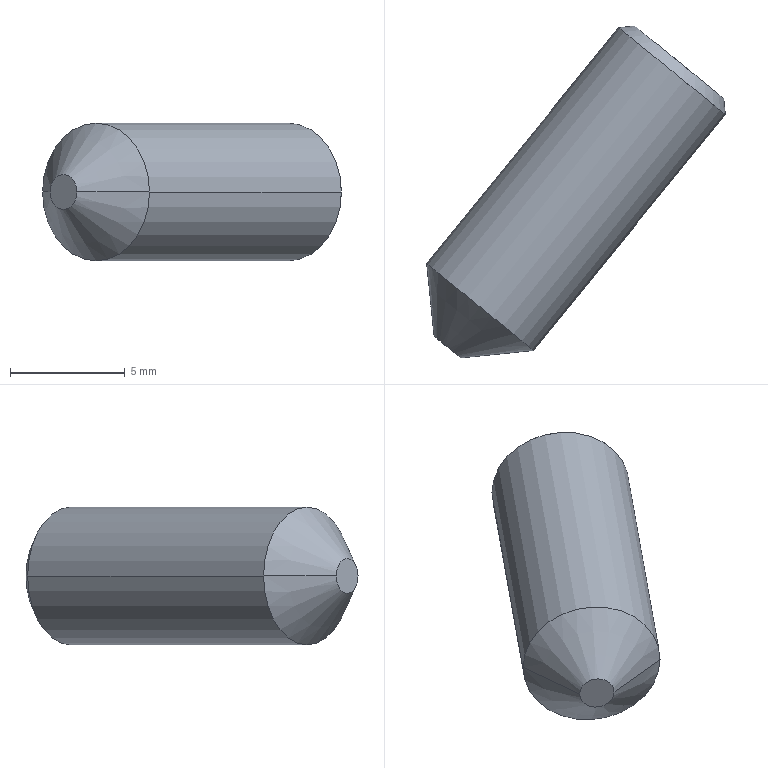Part | SolidWorks | features BaseBody 1 | 1 solid | 16 faces | box 13.015 x 14.464 x 6 mm | volume 387.093 mm3 | plane 10 | cone 4 | cylinder 2 | commonest cylinder face diameters 6 x2
STEP:
#1=CARTESIAN_POINT('',(563.568,-118.862,298.945));
#2=VERTEX_POINT('',#1);
#3=CARTESIAN_POINT('',(558.913,-115.077,298.945));
#4=VERTEX_POINT('',#3);
#5=CARTESIAN_POINT('',(561.241,-116.97,298.945));
#6=DIRECTION('',(-0.6309,-0.7758,0.000000012));
#7=DIRECTION('',(0.7758,-0.6309,0.));
#8=AXIS2_PLACEMENT_3D('',#5,#6,#7);
#9=CIRCLE('',#8,3.);
#10=EDGE_CURVE('',#2,#4,#9,.T.);
#11=ORIENTED_EDGE('',*,*,#10,.T.);
#12=CARTESIAN_POINT('',(550.553,-125.357,298.945));
#13=VERTEX_POINT('',#12);
#14=CARTESIAN_POINT('',(554.733,-120.217,298.945));
#15=DIRECTION('',(-0.6309,-0.7758,0.000000012));
#16=VECTOR('',#15,1000.);
#17=LINE('',#14,#16);
#18=EDGE_CURVE('',#4,#13,#17,.T.);
#19=ORIENTED_EDGE('',*,*,#18,.T.);
#20=CARTESIAN_POINT('',(555.208,-129.142,298.945));
#21=VERTEX_POINT('',#20);
#22=CARTESIAN_POINT('',(552.881,-127.249,298.945));
#23=DIRECTION('',(0.6309,0.7758,-0.000000012));
#24=DIRECTION('',(0.7758,-0.6309,0.));
#25=AXIS2_PLACEMENT_3D('',#22,#23,#24);
#26=CIRCLE('',#25,3.);
#27=EDGE_CURVE('',#13,#21,#26,.T.);
#28=ORIENTED_EDGE('',*,*,#27,.T.);
#29=CARTESIAN_POINT('',(559.388,-124.002,298.945));
#30=DIRECTION('',(-0.6309,-0.7758,0.000000012));
#31=VECTOR('',#30,1000.);
#32=LINE('',#29,#31);
#33=EDGE_CURVE('',#2,#21,#32,.T.);
#34=ORIENTED_EDGE('',*,*,#33,.F.);
#35=EDGE_LOOP('',(#11,#19,#28,#34));
#36=FACE_OUTER_BOUND('',#35,.T.);
#37=CARTESIAN_POINT('',(557.061,-122.109,298.945));
#38=DIRECTION('',(-0.6309,-0.7758,0.000000012));
#39=DIRECTION('',(0.7758,-0.6309,0.));
#40=AXIS2_PLACEMENT_3D('',#37,#38,#39);
#41=CYLINDRICAL_SURFACE('',#40,3.);
#42=ADVANCED_FACE('',(#36),#41,.T.);
#43=CARTESIAN_POINT('',(550.879,-128.522,298.945));
#44=VERTEX_POINT('',#43);
#45=CARTESIAN_POINT('',(552.043,-129.468,298.945));
#46=VERTEX_POINT('',#45);
#47=CARTESIAN_POINT('',(551.461,-128.995,298.945));
#48=DIRECTION('',(0.6309,0.7758,-0.000000012));
#49=DIRECTION('',(-0.7758,0.6309,0.));
#50=AXIS2_PLACEMENT_3D('',#47,#48,#49);
#51=CIRCLE('',#50,0.75);
#52=EDGE_CURVE('',#44,#46,#51,.T.);
#53=ORIENTED_EDGE('',*,*,#52,.T.);
#54=CARTESIAN_POINT('',(555.208,-129.142,298.945));
#55=DIRECTION('',(0.9947,0.1025,-0.000000009));
#56=VECTOR('',#55,1000.);
#57=LINE('',#54,#56);
#58=EDGE_CURVE('',#46,#21,#57,.T.);
#59=ORIENTED_EDGE('',*,*,#58,.T.);
#60=ORIENTED_EDGE('',*,*,#27,.F.);
#61=CARTESIAN_POINT('',(550.553,-125.357,298.945));
#62=DIRECTION('',(-0.1025,0.9947,-0.000000009));
#63=VECTOR('',#62,1000.);
#64=LINE('',#61,#63);
#65=EDGE_CURVE('',#44,#13,#64,.T.);
#66=ORIENTED_EDGE('',*,*,#65,.F.);
#67=EDGE_LOOP('',(#53,#59,#60,#66));
#68=FACE_OUTER_BOUND('',#67,.T.);
#69=CARTESIAN_POINT('',(552.881,-127.249,298.945));
#70=DIRECTION('',(0.6309,0.7758,-0.000000012));
#71=DIRECTION('',(-0.7758,0.6309,0.));
#72=AXIS2_PLACEMENT_3D('',#69,#70,#71);
#73=CONICAL_SURFACE('',#72,3.,0.7854);
#74=ADVANCED_FACE('',(#68),#73,.T.);
#75=CARTESIAN_POINT('',(563.496,-118.159,298.945));
#76=VERTEX_POINT('',#75);
#77=CARTESIAN_POINT('',(559.616,-115.004,298.945));
#78=VERTEX_POINT('',#77);
#79=CARTESIAN_POINT('',(561.556,-116.582,298.945));
#80=DIRECTION('',(-0.6309,-0.7758,0.000000012));
#81=DIRECTION('',(0.7758,-0.6309,0.));
#82=AXIS2_PLACEMENT_3D('',#79,#80,#81);
#83=CIRCLE('',#82,2.5);
#84=EDGE_CURVE('',#76,#78,#83,.T.);
#85=ORIENTED_EDGE('',*,*,#84,.T.);
#86=CARTESIAN_POINT('',(558.914,-115.078,298.945));
#87=VERTEX_POINT('',#86);
#88=CARTESIAN_POINT('',(558.914,-115.078,298.945));
#89=DIRECTION('',(-0.9946,-0.104,0.000000009));
#90=VECTOR('',#89,1000.);
#91=LINE('',#88,#90);
#92=EDGE_CURVE('',#78,#87,#91,.T.);
#93=ORIENTED_EDGE('',*,*,#92,.T.);
#94=CARTESIAN_POINT('',(563.567,-118.861,298.945));
#95=VERTEX_POINT('',#94);
#96=CARTESIAN_POINT('',(561.241,-116.97,298.945));
#97=DIRECTION('',(-0.6309,-0.7758,0.000000012));
#98=DIRECTION('',(0.7758,-0.6309,0.));
#99=AXIS2_PLACEMENT_3D('',#96,#97,#98);
#100=CIRCLE('',#99,2.998);
#101=EDGE_CURVE('',#95,#87,#100,.T.);
#102=ORIENTED_EDGE('',*,*,#101,.F.);
#103=CARTESIAN_POINT('',(563.567,-118.861,298.945));
#104=DIRECTION('',(0.101,-0.9949,0.000000009));
#105=VECTOR('',#104,1000.);
#106=LINE('',#103,#105);
#107=EDGE_CURVE('',#76,#95,#106,.T.);
#108=ORIENTED_EDGE('',*,*,#107,.F.);
#109=EDGE_LOOP('',(#85,#93,#102,#108));
#110=FACE_OUTER_BOUND('',#109,.T.);
#111=CARTESIAN_POINT('',(561.241,-116.97,298.945));
#112=DIRECTION('',(-0.6309,-0.7758,0.000000012));
#113=DIRECTION('',(0.7758,-0.6309,0.));
#114=AXIS2_PLACEMENT_3D('',#111,#112,#113);
#115=CONICAL_SURFACE('',#114,2.998,0.7839);
#116=ADVANCED_FACE('',(#110),#115,.T.);
#117=ORIENTED_EDGE('',*,*,#18,.F.);
#118=CARTESIAN_POINT('',(561.241,-116.97,295.945));
#119=VERTEX_POINT('',#118);
#120=CARTESIAN_POINT('',(561.241,-116.97,298.945));
#121=DIRECTION('',(-0.6309,-0.7758,0.000000012));
#122=DIRECTION('',(0.7758,-0.6309,0.));
#123=AXIS2_PLACEMENT_3D('',#120,#121,#122);
#124=CIRCLE('',#123,3.);
#125=EDGE_CURVE('',#4,#119,#124,.T.);
#126=ORIENTED_EDGE('',*,*,#125,.T.);
#127=CARTESIAN_POINT('',(561.241,-116.97,298.945));
#128=DIRECTION('',(-0.6309,-0.7758,0.000000012));
#129=DIRECTION('',(0.7758,-0.6309,0.));
#130=AXIS2_PLACEMENT_3D('',#127,#128,#129);
#131=CIRCLE('',#130,3.);
#132=EDGE_CURVE('',#119,#2,#131,.T.);
#133=ORIENTED_EDGE('',*,*,#132,.T.);
#134=ORIENTED_EDGE('',*,*,#33,.T.);
#135=CARTESIAN_POINT('',(552.881,-127.249,298.945));
#136=DIRECTION('',(0.6309,0.7758,-0.000000012));
#137=DIRECTION('',(0.7758,-0.6309,0.));
#138=AXIS2_PLACEMENT_3D('',#135,#136,#137);
#139=CIRCLE('',#138,3.);
#140=EDGE_CURVE('',#21,#13,#139,.T.);
#141=ORIENTED_EDGE('',*,*,#140,.T.);
#142=EDGE_LOOP('',(#117,#126,#133,#134,#141));
#143=FACE_OUTER_BOUND('',#142,.T.);
#144=CARTESIAN_POINT('',(557.061,-122.109,298.945));
#145=DIRECTION('',(-0.6309,-0.7758,0.000000012));
#146=DIRECTION('',(0.7758,-0.6309,0.));
#147=AXIS2_PLACEMENT_3D('',#144,#145,#146);
#148=CYLINDRICAL_SURFACE('',#147,3.);
#149=ADVANCED_FACE('',(#143),#148,.T.);
#150=ORIENTED_EDGE('',*,*,#132,.F.);
#151=CARTESIAN_POINT('',(561.241,-116.97,298.945));
#152=DIRECTION('',(-0.6309,-0.7758,0.000000012));
#153=DIRECTION('',(0.7758,-0.6309,0.));
#154=AXIS2_PLACEMENT_3D('',#151,#152,#153);
#155=CIRCLE('',#154,2.998);
#156=EDGE_CURVE('',#119,#95,#155,.T.);
#157=ORIENTED_EDGE('',*,*,#156,.T.);
#158=ORIENTED_EDGE('',*,*,#101,.T.);
#159=CARTESIAN_POINT('',(561.241,-116.97,298.945));
#160=DIRECTION('',(-0.6309,-0.7758,0.000000012));
#161=DIRECTION('',(0.7758,-0.6309,0.));
#162=AXIS2_PLACEMENT_3D('',#159,#160,#161);
#163=CIRCLE('',#162,2.998);
#164=EDGE_CURVE('',#87,#119,#163,.T.);
#165=ORIENTED_EDGE('',*,*,#164,.T.);
#166=ORIENTED_EDGE('',*,*,#125,.F.);
#167=ORIENTED_EDGE('',*,*,#10,.F.);
#168=EDGE_LOOP('',(#150,#157,#158,#165,#166,#167));
#169=FACE_OUTER_BOUND('',#168,.T.);
#170=CARTESIAN_POINT('',(561.241,-116.97,295.945));
#171=DIRECTION('',(0.6309,0.7758,-0.000000012));
#172=DIRECTION('',(-0.7758,0.6309,0.));
#173=AXIS2_PLACEMENT_3D('',#170,#171,#172);
#174=PLANE('',#173);
#175=ADVANCED_FACE('',(#169),#174,.T.);
#176=ORIENTED_EDGE('',*,*,#58,.F.);
#177=CARTESIAN_POINT('',(551.461,-128.995,298.945));
#178=DIRECTION('',(0.6309,0.7758,-0.000000012));
#179=DIRECTION('',(-0.7758,0.6309,0.));
#180=AXIS2_PLACEMENT_3D('',#177,#178,#179);
#181=CIRCLE('',#180,0.75);
#182=EDGE_CURVE('',#46,#44,#181,.T.);
#183=ORIENTED_EDGE('',*,*,#182,.T.);
#184=ORIENTED_EDGE('',*,*,#65,.T.);
#185=ORIENTED_EDGE('',*,*,#140,.F.);
#186=EDGE_LOOP('',(#176,#183,#184,#185));
#187=FACE_OUTER_BOUND('',#186,.T.);
#188=CARTESIAN_POINT('',(552.881,-127.249,298.945));
#189=DIRECTION('',(0.6309,0.7758,-0.000000012));
#190=DIRECTION('',(-0.7758,0.6309,0.));
#191=AXIS2_PLACEMENT_3D('',#188,#189,#190);
#192=CONICAL_SURFACE('',#191,3.,0.7854);
#193=ADVANCED_FACE('',(#187),#192,.T.);
#194=ORIENTED_EDGE('',*,*,#92,.F.);
#195=CARTESIAN_POINT('',(561.556,-116.582,298.945));
#196=DIRECTION('',(-0.6309,-0.7758,0.000000012));
#197=DIRECTION('',(0.7758,-0.6309,0.));
#198=AXIS2_PLACEMENT_3D('',#195,#196,#197);
#199=CIRCLE('',#198,2.5);
#200=EDGE_CURVE('',#78,#76,#199,.T.);
#201=ORIENTED_EDGE('',*,*,#200,.T.);
#202=ORIENTED_EDGE('',*,*,#107,.T.);
#203=ORIENTED_EDGE('',*,*,#156,.F.);
#204=ORIENTED_EDGE('',*,*,#164,.F.);
#205=EDGE_LOOP('',(#194,#201,#202,#203,#204));
#206=FACE_OUTER_BOUND('',#205,.T.);
#207=CARTESIAN_POINT('',(561.241,-116.97,298.945));
#208=DIRECTION('',(-0.6309,-0.7758,0.000000012));
#209=DIRECTION('',(0.7758,-0.6309,0.));
#210=AXIS2_PLACEMENT_3D('',#207,#208,#209);
#211=CONICAL_SURFACE('',#210,2.998,0.7839);
#212=ADVANCED_FACE('',(#206),#211,.T.);
#213=ORIENTED_EDGE('',*,*,#52,.F.);
#214=ORIENTED_EDGE('',*,*,#182,.F.);
#215=EDGE_LOOP('',(#213,#214));
#216=FACE_OUTER_BOUND('',#215,.T.);
#217=CARTESIAN_POINT('',(551.461,-128.995,298.57));
#218=DIRECTION('',(-0.6309,-0.7758,0.000000012));
#219=DIRECTION('',(0.7758,-0.6309,0.));
#220=AXIS2_PLACEMENT_3D('',#217,#218,#219);
#221=PLANE('',#220);
#222=ADVANCED_FACE('',(#216),#221,.T.);
#223=ORIENTED_EDGE('',*,*,#84,.F.);
#224=ORIENTED_EDGE('',*,*,#200,.F.);
#225=EDGE_LOOP('',(#223,#224));
#226=FACE_OUTER_BOUND('',#225,.T.);
#227=CARTESIAN_POINT('',(562.72,-117.528,299.811));
#228=VERTEX_POINT('',#227);
#229=CARTESIAN_POINT('',(561.556,-116.582,300.677));
#230=VERTEX_POINT('',#229);
#231=CARTESIAN_POINT('',(562.72,-117.528,299.811));
#232=DIRECTION('',(-0.6719,0.5464,0.5));
#233=VECTOR('',#232,1000.);
#234=LINE('',#231,#233);
#235=EDGE_CURVE('',#228,#230,#234,.T.);
#236=ORIENTED_EDGE('',*,*,#235,.T.);
#237=CARTESIAN_POINT('',(560.392,-115.635,299.811));
#238=VERTEX_POINT('',#237);
#239=CARTESIAN_POINT('',(561.556,-116.582,300.677));
#240=DIRECTION('',(-0.6719,0.5464,-0.5));
#241=VECTOR('',#240,1000.);
#242=LINE('',#239,#241);
#243=EDGE_CURVE('',#230,#238,#242,.T.);
#244=ORIENTED_EDGE('',*,*,#243,.T.);
#245=CARTESIAN_POINT('',(560.392,-115.635,298.079));
#246=VERTEX_POINT('',#245);
#247=CARTESIAN_POINT('',(560.392,-115.635,298.079));
#248=DIRECTION('',(-0.000000028,0.000000023,-1.));
#249=VECTOR('',#248,1000.);
#250=LINE('',#247,#249);
#251=EDGE_CURVE('',#238,#246,#250,.T.);
#252=ORIENTED_EDGE('',*,*,#251,.T.);
#253=CARTESIAN_POINT('',(561.556,-116.582,297.213));
#254=VERTEX_POINT('',#253);
#255=CARTESIAN_POINT('',(560.392,-115.635,298.079));
#256=DIRECTION('',(0.6719,-0.5464,-0.5));
#257=VECTOR('',#256,1000.);
#258=LINE('',#255,#257);
#259=EDGE_CURVE('',#246,#254,#258,.T.);
#260=ORIENTED_EDGE('',*,*,#259,.T.);
#261=CARTESIAN_POINT('',(562.72,-117.528,298.079));
#262=VERTEX_POINT('',#261);
#263=CARTESIAN_POINT('',(561.556,-116.582,297.213));
#264=DIRECTION('',(0.6719,-0.5464,0.5));
#265=VECTOR('',#264,1000.);
#266=LINE('',#263,#265);
#267=EDGE_CURVE('',#254,#262,#266,.T.);
#268=ORIENTED_EDGE('',*,*,#267,.T.);
#269=CARTESIAN_POINT('',(562.72,-117.528,299.811));
#270=DIRECTION('',(0.000000028,-0.000000023,1.));
#271=VECTOR('',#270,1000.);
#272=LINE('',#269,#271);
#273=EDGE_CURVE('',#262,#228,#272,.T.);
#274=ORIENTED_EDGE('',*,*,#273,.T.);
#275=EDGE_LOOP('',(#236,#244,#252,#260,#268,#274));
#276=FACE_BOUND('',#275,.T.);
#277=CARTESIAN_POINT('',(561.556,-116.582,297.695));
#278=DIRECTION('',(0.6309,0.7758,-0.000000012));
#279=DIRECTION('',(-0.7758,0.6309,0.));
#280=AXIS2_PLACEMENT_3D('',#277,#278,#279);
#281=PLANE('',#280);
#282=ADVANCED_FACE('',(#226,#276),#281,.T.);
#283=CARTESIAN_POINT('',(558.184,-118.351,299.811));
#284=VERTEX_POINT('',#283);
#285=CARTESIAN_POINT('',(560.392,-115.635,299.811));
#286=DIRECTION('',(-0.6309,-0.7758,0.000000012));
#287=VECTOR('',#286,1000.);
#288=LINE('',#285,#287);
#289=EDGE_CURVE('',#238,#284,#288,.T.);
#290=ORIENTED_EDGE('',*,*,#289,.F.);
#291=ORIENTED_EDGE('',*,*,#243,.F.);
#292=CARTESIAN_POINT('',(559.348,-119.297,300.677));
#293=VERTEX_POINT('',#292);
#294=CARTESIAN_POINT('',(559.348,-119.297,300.677));
#295=DIRECTION('',(0.6309,0.7758,-0.000000012));
#296=VECTOR('',#295,1000.);
#297=LINE('',#294,#296);
#298=EDGE_CURVE('',#293,#230,#297,.T.);
#299=ORIENTED_EDGE('',*,*,#298,.F.);
#300=CARTESIAN_POINT('',(558.184,-118.351,299.811));
#301=DIRECTION('',(0.6719,-0.5464,0.5));
#302=VECTOR('',#301,1000.);
#303=LINE('',#300,#302);
#304=EDGE_CURVE('',#284,#293,#303,.T.);
#305=ORIENTED_EDGE('',*,*,#304,.F.);
#306=EDGE_LOOP('',(#290,#291,#299,#305));
#307=FACE_OUTER_BOUND('',#306,.T.);
#308=CARTESIAN_POINT('',(560.392,-115.635,299.811));
#309=DIRECTION('',(-0.3879,0.3155,0.866));
#310=DIRECTION('',(0.9126,0.,0.4088));
#311=AXIS2_PLACEMENT_3D('',#308,#309,#310);
#312=PLANE('',#311);
#313=ADVANCED_FACE('',(#307),#312,.F.);
#314=CARTESIAN_POINT('',(560.512,-120.243,298.079));
#315=VERTEX_POINT('',#314);
#316=CARTESIAN_POINT('',(559.348,-119.297,297.213));
#317=VERTEX_POINT('',#316);
#318=CARTESIAN_POINT('',(560.512,-120.243,298.079));
#319=DIRECTION('',(-0.6719,0.5464,-0.5));
#320=VECTOR('',#319,1000.);
#321=LINE('',#318,#320);
#322=EDGE_CURVE('',#315,#317,#321,.T.);
#323=ORIENTED_EDGE('',*,*,#322,.T.);
#324=CARTESIAN_POINT('',(558.184,-118.351,298.079));
#325=VERTEX_POINT('',#324);
#326=CARTESIAN_POINT('',(559.348,-119.297,297.213));
#327=DIRECTION('',(-0.6719,0.5464,0.5));
#328=VECTOR('',#327,1000.);
#329=LINE('',#326,#328);
#330=EDGE_CURVE('',#317,#325,#329,.T.);
#331=ORIENTED_EDGE('',*,*,#330,.T.);
#332=CARTESIAN_POINT('',(558.184,-118.351,298.945));
#333=DIRECTION('',(0.000000008,0.000000009,1.));
#334=VECTOR('',#333,1000.);
#335=LINE('',#332,#334);
#336=EDGE_CURVE('',#325,#284,#335,.T.);
#337=ORIENTED_EDGE('',*,*,#336,.T.);
#338=ORIENTED_EDGE('',*,*,#304,.T.);
#339=CARTESIAN_POINT('',(560.512,-120.243,299.811));
#340=VERTEX_POINT('',#339);
#341=CARTESIAN_POINT('',(559.348,-119.297,300.677));
#342=DIRECTION('',(0.6719,-0.5464,-0.5));
#343=VECTOR('',#342,1000.);
#344=LINE('',#341,#343);
#345=EDGE_CURVE('',#293,#340,#344,.T.);
#346=ORIENTED_EDGE('',*,*,#345,.T.);
#347=CARTESIAN_POINT('',(560.512,-120.243,299.811));
#348=DIRECTION('',(-0.000000028,0.000000023,-1.));
#349=VECTOR('',#348,1000.);
#350=LINE('',#347,#349);
#351=EDGE_CURVE('',#340,#315,#350,.T.);
#352=ORIENTED_EDGE('',*,*,#351,.T.);
#353=EDGE_LOOP('',(#323,#331,#337,#338,#346,#352));
#354=FACE_OUTER_BOUND('',#353,.T.);
#355=CARTESIAN_POINT('',(559.348,-119.297,298.945));
#356=DIRECTION('',(0.6309,0.7758,-0.000000012));
#357=DIRECTION('',(-0.7758,0.6309,0.));
#358=AXIS2_PLACEMENT_3D('',#355,#356,#357);
#359=PLANE('',#358);
#360=ADVANCED_FACE('',(#354),#359,.T.);
#361=CARTESIAN_POINT('',(560.392,-115.635,298.079));
#362=DIRECTION('',(-0.6309,-0.7758,0.));
#363=VECTOR('',#362,1000.);
#364=LINE('',#361,#363);
#365=EDGE_CURVE('',#246,#325,#364,.T.);
#366=ORIENTED_EDGE('',*,*,#365,.F.);
#367=ORIENTED_EDGE('',*,*,#251,.F.);
#368=ORIENTED_EDGE('',*,*,#289,.T.);
#369=ORIENTED_EDGE('',*,*,#336,.F.);
#370=EDGE_LOOP('',(#366,#367,#368,#369));
#371=FACE_OUTER_BOUND('',#370,.T.);
#372=CARTESIAN_POINT('',(560.392,-115.635,298.079));
#373=DIRECTION('',(-0.7758,0.6309,0.000000036));
#374=DIRECTION('',(-0.6309,-0.7758,0.));
#375=AXIS2_PLACEMENT_3D('',#372,#373,#374);
#376=PLANE('',#375);
#377=ADVANCED_FACE('',(#371),#376,.F.);
#378=ORIENTED_EDGE('',*,*,#298,.T.);
#379=ORIENTED_EDGE('',*,*,#235,.F.);
#380=CARTESIAN_POINT('',(560.512,-120.243,299.811));
#381=DIRECTION('',(0.6309,0.7758,-0.000000012));
#382=VECTOR('',#381,1000.);
#383=LINE('',#380,#382);
#384=EDGE_CURVE('',#340,#228,#383,.T.);
#385=ORIENTED_EDGE('',*,*,#384,.F.);
#386=ORIENTED_EDGE('',*,*,#345,.F.);
#387=EDGE_LOOP('',(#378,#379,#385,#386));
#388=FACE_OUTER_BOUND('',#387,.T.);
#389=CARTESIAN_POINT('',(561.556,-116.582,300.677));
#390=DIRECTION('',(0.3879,-0.3155,0.866));
#391=DIRECTION('',(0.9126,0.,-0.4088));
#392=AXIS2_PLACEMENT_3D('',#389,#390,#391);
#393=PLANE('',#392);
#394=ADVANCED_FACE('',(#388),#393,.F.);
#395=CARTESIAN_POINT('',(561.556,-116.582,297.213));
#396=DIRECTION('',(-0.6309,-0.7758,0.000000012));
#397=VECTOR('',#396,1000.);
#398=LINE('',#395,#397);
#399=EDGE_CURVE('',#254,#317,#398,.T.);
#400=ORIENTED_EDGE('',*,*,#399,.F.);
#401=ORIENTED_EDGE('',*,*,#259,.F.);
#402=ORIENTED_EDGE('',*,*,#365,.T.);
#403=ORIENTED_EDGE('',*,*,#330,.F.);
#404=EDGE_LOOP('',(#400,#401,#402,#403));
#405=FACE_OUTER_BOUND('',#404,.T.);
#406=CARTESIAN_POINT('',(561.556,-116.582,297.213));
#407=DIRECTION('',(-0.3879,0.3155,-0.866));
#408=DIRECTION('',(-0.9126,0.,0.4088));
#409=AXIS2_PLACEMENT_3D('',#406,#407,#408);
#410=PLANE('',#409);
#411=ADVANCED_FACE('',(#405),#410,.F.);
#412=ORIENTED_EDGE('',*,*,#384,.T.);
#413=ORIENTED_EDGE('',*,*,#273,.F.);
#414=CARTESIAN_POINT('',(562.72,-117.528,298.079));
#415=DIRECTION('',(0.6309,0.7758,0.));
#416=VECTOR('',#415,1000.);
#417=LINE('',#414,#416);
#418=EDGE_CURVE('',#315,#262,#417,.T.);
#419=ORIENTED_EDGE('',*,*,#418,.F.);
#420=ORIENTED_EDGE('',*,*,#351,.F.);
#421=EDGE_LOOP('',(#412,#413,#419,#420));
#422=FACE_OUTER_BOUND('',#421,.T.);
#423=CARTESIAN_POINT('',(562.72,-117.528,299.811));
#424=DIRECTION('',(0.7758,-0.6309,-0.000000036));
#425=DIRECTION('',(0.6309,0.7758,0.));
#426=AXIS2_PLACEMENT_3D('',#423,#424,#425);
#427=PLANE('',#426);
#428=ADVANCED_FACE('',(#422),#427,.F.);
#429=ORIENTED_EDGE('',*,*,#418,.T.);
#430=ORIENTED_EDGE('',*,*,#267,.F.);
#431=ORIENTED_EDGE('',*,*,#399,.T.);
#432=ORIENTED_EDGE('',*,*,#322,.F.);
#433=EDGE_LOOP('',(#429,#430,#431,#432));
#434=FACE_OUTER_BOUND('',#433,.T.);
#435=CARTESIAN_POINT('',(562.72,-117.528,298.079));
#436=DIRECTION('',(0.3879,-0.3155,-0.866));
#437=DIRECTION('',(-0.9126,0.,-0.4088));
#438=AXIS2_PLACEMENT_3D('',#435,#436,#437);
#439=PLANE('',#438);
#440=ADVANCED_FACE('',(#434),#439,.F.);
#441=CLOSED_SHELL('',(#42,#74,#116,#149,#175,#193,#212,#222,#282,#313,#360,#377,#394,#411,#428,#440));
#442=MANIFOLD_SOLID_BREP('',#441);
#443=CARTESIAN_POINT('',(0.,0.,0.));
#444=DIRECTION('',(0.,0.,1.));
#445=DIRECTION('',(1.,0.,0.));
#446=AXIS2_PLACEMENT_3D('',#443,#444,#445);
#447=(LENGTH_UNIT()NAMED_UNIT(*)SI_UNIT(.MILLI.,.METRE.));
#448=UNCERTAINTY_MEASURE_WITH_UNIT(LENGTH_MEASURE(0.00001),#447,'','');
#449=(NAMED_UNIT(*)PLANE_ANGLE_UNIT()SI_UNIT($,.RADIAN.));
#450=(NAMED_UNIT(*)SI_UNIT($,.STERADIAN.)SOLID_ANGLE_UNIT());
#451=(GEOMETRIC_REPRESENTATION_CONTEXT(3)GLOBAL_UNCERTAINTY_ASSIGNED_CONTEXT((#448))GLOBAL_UNIT_ASSIGNED_CONTEXT((#447,#449,#450))REPRESENTATION_CONTEXT('',''));
#452=ADVANCED_BREP_SHAPE_REPRESENTATION('',(#442,#446),#451);